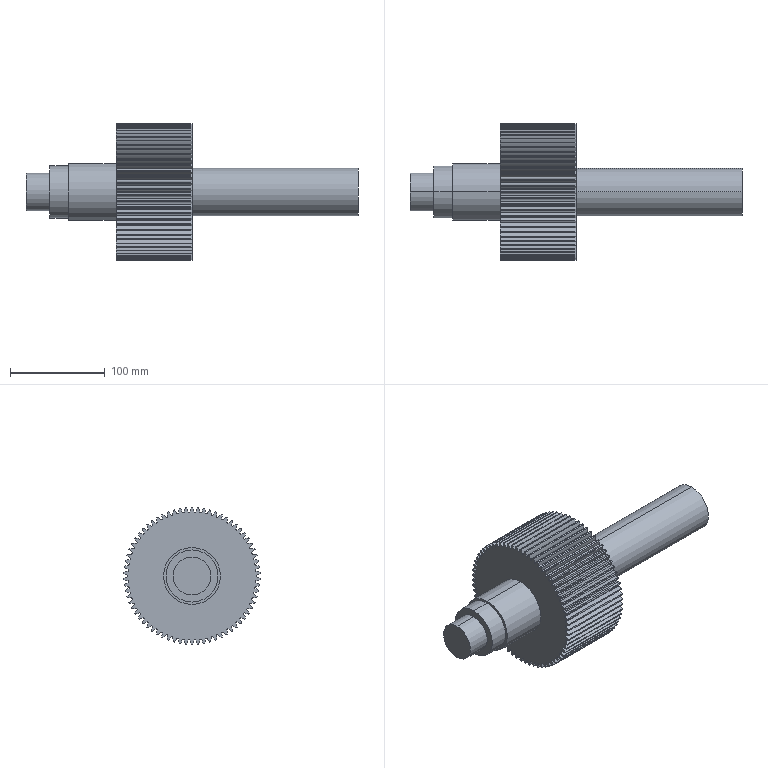Part | SolidWorks | features ICE 4, Boss 3, Cut 3, CirPattern 2, Fillet 2, Revolution 1 | 1 solid | 303 faces | box 350 x 143.909 x 144 mm | volume 1783229 mm3 | cylinder 295 | plane 8 | commonest cylinder face diameters 56 x144 144 x71 134.998 x70 5 x2 40 x2 50 x2